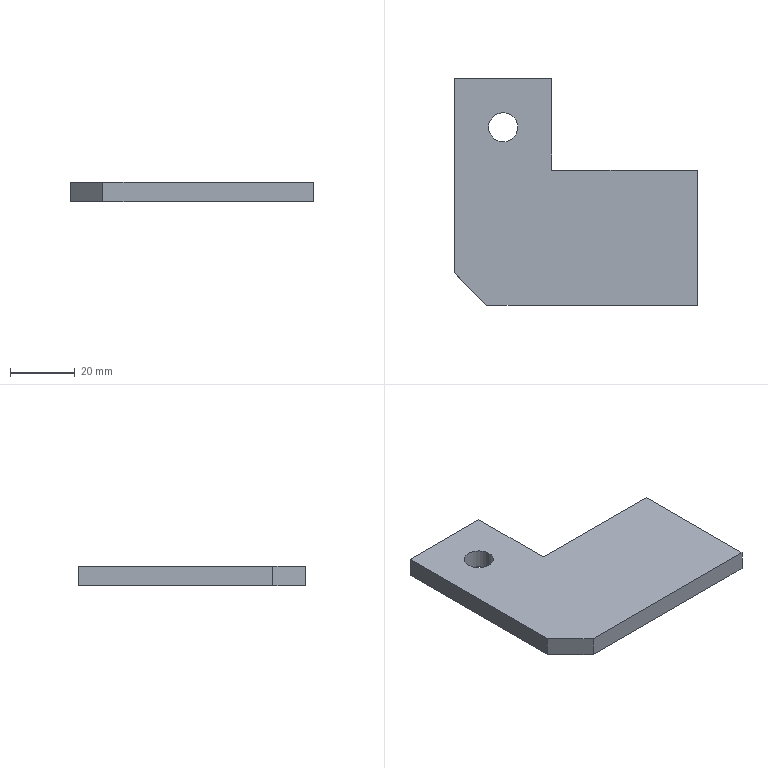Part | SolidWorks | features Chamfer 1, Extrusion 1, ICE 1 | 1 solid | 11 faces | box 75 x 70 x 6 mm | volume 23195 mm3 | plane 9 | cylinder 2 | commonest cylinder face diameters 9 x2
STEP:
#1=CARTESIAN_POINT('',(-23.022,36.378,0.));
#2=VERTEX_POINT('',#1);
#3=CARTESIAN_POINT('',(-14.022,36.378,0.));
#4=VERTEX_POINT('',#3);
#5=CARTESIAN_POINT('',(-18.522,36.378,0.));
#6=DIRECTION('',(0.,0.,1.));
#7=DIRECTION('',(-1.,0.,0.));
#8=AXIS2_PLACEMENT_3D('',#5,#6,#7);
#9=CIRCLE('',#8,4.5);
#10=EDGE_CURVE('',#2,#4,#9,.T.);
#11=ORIENTED_EDGE('',*,*,#10,.F.);
#12=CARTESIAN_POINT('',(-23.022,36.378,6.));
#13=VERTEX_POINT('',#12);
#14=CARTESIAN_POINT('',(-23.022,36.378,-0.001));
#15=DIRECTION('',(0.,0.,1.));
#16=VECTOR('',#15,1000.);
#17=LINE('',#14,#16);
#18=EDGE_CURVE('',#2,#13,#17,.T.);
#19=ORIENTED_EDGE('',*,*,#18,.T.);
#20=CARTESIAN_POINT('',(-14.022,36.378,6.));
#21=VERTEX_POINT('',#20);
#22=CARTESIAN_POINT('',(-18.522,36.378,6.));
#23=DIRECTION('',(0.,0.,1.));
#24=DIRECTION('',(1.,0.,0.));
#25=AXIS2_PLACEMENT_3D('',#22,#23,#24);
#26=CIRCLE('',#25,4.5);
#27=EDGE_CURVE('',#13,#21,#26,.T.);
#28=ORIENTED_EDGE('',*,*,#27,.T.);
#29=CARTESIAN_POINT('',(-14.022,36.378,-0.001));
#30=DIRECTION('',(0.,0.,1.));
#31=VECTOR('',#30,1000.);
#32=LINE('',#29,#31);
#33=EDGE_CURVE('',#4,#21,#32,.T.);
#34=ORIENTED_EDGE('',*,*,#33,.F.);
#35=EDGE_LOOP('',(#11,#19,#28,#34));
#36=FACE_OUTER_BOUND('',#35,.T.);
#37=CARTESIAN_POINT('',(-18.522,36.378,-0.001));
#38=DIRECTION('',(0.,0.,1.));
#39=DIRECTION('',(1.,0.,0.));
#40=AXIS2_PLACEMENT_3D('',#37,#38,#39);
#41=CYLINDRICAL_SURFACE('',#40,4.5);
#42=ADVANCED_FACE('',(#36),#41,.F.);
#43=CARTESIAN_POINT('',(-23.522,-18.622,6.));
#44=VERTEX_POINT('',#43);
#45=CARTESIAN_POINT('',(41.478,-18.622,6.));
#46=VERTEX_POINT('',#45);
#47=CARTESIAN_POINT('',(41.478,-18.622,6.));
#48=DIRECTION('',(1.,0.,0.));
#49=VECTOR('',#48,1000.);
#50=LINE('',#47,#49);
#51=EDGE_CURVE('',#44,#46,#50,.T.);
#52=ORIENTED_EDGE('',*,*,#51,.F.);
#53=CARTESIAN_POINT('',(-23.522,-18.622,0.));
#54=VERTEX_POINT('',#53);
#55=CARTESIAN_POINT('',(-23.522,-18.622,6.));
#56=DIRECTION('',(0.,0.,-1.));
#57=VECTOR('',#56,1000.);
#58=LINE('',#55,#57);
#59=EDGE_CURVE('',#44,#54,#58,.T.);
#60=ORIENTED_EDGE('',*,*,#59,.T.);
#61=CARTESIAN_POINT('',(41.478,-18.622,0.));
#62=VERTEX_POINT('',#61);
#63=CARTESIAN_POINT('',(41.478,-18.622,0.));
#64=DIRECTION('',(1.,0.,0.));
#65=VECTOR('',#64,1000.);
#66=LINE('',#63,#65);
#67=EDGE_CURVE('',#54,#62,#66,.T.);
#68=ORIENTED_EDGE('',*,*,#67,.T.);
#69=CARTESIAN_POINT('',(41.478,-18.622,6.));
#70=DIRECTION('',(0.,0.,-1.));
#71=VECTOR('',#70,1000.);
#72=LINE('',#69,#71);
#73=EDGE_CURVE('',#46,#62,#72,.T.);
#74=ORIENTED_EDGE('',*,*,#73,.F.);
#75=EDGE_LOOP('',(#52,#60,#68,#74));
#76=FACE_OUTER_BOUND('',#75,.T.);
#77=CARTESIAN_POINT('',(41.478,-18.622,6.));
#78=DIRECTION('',(0.,1.,0.));
#79=DIRECTION('',(-1.,0.,0.));
#80=AXIS2_PLACEMENT_3D('',#77,#78,#79);
#81=PLANE('',#80);
#82=ADVANCED_FACE('',(#76),#81,.F.);
#83=CARTESIAN_POINT('',(41.478,23.145,0.));
#84=VERTEX_POINT('',#83);
#85=CARTESIAN_POINT('',(41.478,23.145,0.));
#86=DIRECTION('',(0.,1.,0.));
#87=VECTOR('',#86,1000.);
#88=LINE('',#85,#87);
#89=EDGE_CURVE('',#62,#84,#88,.T.);
#90=ORIENTED_EDGE('',*,*,#89,.T.);
#91=CARTESIAN_POINT('',(41.478,23.145,6.));
#92=VERTEX_POINT('',#91);
#93=CARTESIAN_POINT('',(41.478,23.145,6.));
#94=DIRECTION('',(0.,0.,-1.));
#95=VECTOR('',#94,1000.);
#96=LINE('',#93,#95);
#97=EDGE_CURVE('',#92,#84,#96,.T.);
#98=ORIENTED_EDGE('',*,*,#97,.F.);
#99=CARTESIAN_POINT('',(41.478,23.145,6.));
#100=DIRECTION('',(0.,1.,0.));
#101=VECTOR('',#100,1000.);
#102=LINE('',#99,#101);
#103=EDGE_CURVE('',#46,#92,#102,.T.);
#104=ORIENTED_EDGE('',*,*,#103,.F.);
#105=ORIENTED_EDGE('',*,*,#73,.T.);
#106=EDGE_LOOP('',(#90,#98,#104,#105));
#107=FACE_OUTER_BOUND('',#106,.T.);
#108=CARTESIAN_POINT('',(41.478,23.145,6.));
#109=DIRECTION('',(-1.,0.,0.));
#110=DIRECTION('',(0.,0.,1.));
#111=AXIS2_PLACEMENT_3D('',#108,#109,#110);
#112=PLANE('',#111);
#113=ADVANCED_FACE('',(#107),#112,.F.);
#114=CARTESIAN_POINT('',(-3.522,23.145,0.));
#115=VERTEX_POINT('',#114);
#116=CARTESIAN_POINT('',(-3.522,23.145,0.));
#117=DIRECTION('',(-1.,0.,0.));
#118=VECTOR('',#117,1000.);
#119=LINE('',#116,#118);
#120=EDGE_CURVE('',#84,#115,#119,.T.);
#121=ORIENTED_EDGE('',*,*,#120,.T.);
#122=CARTESIAN_POINT('',(-3.522,23.145,6.));
#123=VERTEX_POINT('',#122);
#124=CARTESIAN_POINT('',(-3.522,23.145,6.));
#125=DIRECTION('',(0.,0.,-1.));
#126=VECTOR('',#125,1000.);
#127=LINE('',#124,#126);
#128=EDGE_CURVE('',#123,#115,#127,.T.);
#129=ORIENTED_EDGE('',*,*,#128,.F.);
#130=CARTESIAN_POINT('',(-3.522,23.145,6.));
#131=DIRECTION('',(-1.,0.,0.));
#132=VECTOR('',#131,1000.);
#133=LINE('',#130,#132);
#134=EDGE_CURVE('',#92,#123,#133,.T.);
#135=ORIENTED_EDGE('',*,*,#134,.F.);
#136=ORIENTED_EDGE('',*,*,#97,.T.);
#137=EDGE_LOOP('',(#121,#129,#135,#136));
#138=FACE_OUTER_BOUND('',#137,.T.);
#139=CARTESIAN_POINT('',(-3.522,23.145,6.));
#140=DIRECTION('',(0.,-1.,0.));
#141=DIRECTION('',(0.,0.,-1.));
#142=AXIS2_PLACEMENT_3D('',#139,#140,#141);
#143=PLANE('',#142);
#144=ADVANCED_FACE('',(#138),#143,.F.);
#145=CARTESIAN_POINT('',(-3.522,51.378,0.));
#146=VERTEX_POINT('',#145);
#147=CARTESIAN_POINT('',(-3.522,51.378,0.));
#148=DIRECTION('',(0.,1.,0.));
#149=VECTOR('',#148,1000.);
#150=LINE('',#147,#149);
#151=EDGE_CURVE('',#115,#146,#150,.T.);
#152=ORIENTED_EDGE('',*,*,#151,.T.);
#153=CARTESIAN_POINT('',(-3.522,51.378,6.));
#154=VERTEX_POINT('',#153);
#155=CARTESIAN_POINT('',(-3.522,51.378,6.));
#156=DIRECTION('',(0.,0.,-1.));
#157=VECTOR('',#156,1000.);
#158=LINE('',#155,#157);
#159=EDGE_CURVE('',#154,#146,#158,.T.);
#160=ORIENTED_EDGE('',*,*,#159,.F.);
#161=CARTESIAN_POINT('',(-3.522,51.378,6.));
#162=DIRECTION('',(0.,1.,0.));
#163=VECTOR('',#162,1000.);
#164=LINE('',#161,#163);
#165=EDGE_CURVE('',#123,#154,#164,.T.);
#166=ORIENTED_EDGE('',*,*,#165,.F.);
#167=ORIENTED_EDGE('',*,*,#128,.T.);
#168=EDGE_LOOP('',(#152,#160,#166,#167));
#169=FACE_OUTER_BOUND('',#168,.T.);
#170=CARTESIAN_POINT('',(-3.522,51.378,6.));
#171=DIRECTION('',(-1.,0.,0.));
#172=DIRECTION('',(0.,-1.,0.));
#173=AXIS2_PLACEMENT_3D('',#170,#171,#172);
#174=PLANE('',#173);
#175=ADVANCED_FACE('',(#169),#174,.F.);
#176=CARTESIAN_POINT('',(-33.522,51.378,0.));
#177=VERTEX_POINT('',#176);
#178=CARTESIAN_POINT('',(-33.522,51.378,0.));
#179=DIRECTION('',(-1.,0.,0.));
#180=VECTOR('',#179,1000.);
#181=LINE('',#178,#180);
#182=EDGE_CURVE('',#146,#177,#181,.T.);
#183=ORIENTED_EDGE('',*,*,#182,.T.);
#184=CARTESIAN_POINT('',(-33.522,51.378,6.));
#185=VERTEX_POINT('',#184);
#186=CARTESIAN_POINT('',(-33.522,51.378,6.));
#187=DIRECTION('',(0.,0.,-1.));
#188=VECTOR('',#187,1000.);
#189=LINE('',#186,#188);
#190=EDGE_CURVE('',#185,#177,#189,.T.);
#191=ORIENTED_EDGE('',*,*,#190,.F.);
#192=CARTESIAN_POINT('',(-33.522,51.378,6.));
#193=DIRECTION('',(-1.,0.,0.));
#194=VECTOR('',#193,1000.);
#195=LINE('',#192,#194);
#196=EDGE_CURVE('',#154,#185,#195,.T.);
#197=ORIENTED_EDGE('',*,*,#196,.F.);
#198=ORIENTED_EDGE('',*,*,#159,.T.);
#199=EDGE_LOOP('',(#183,#191,#197,#198));
#200=FACE_OUTER_BOUND('',#199,.T.);
#201=CARTESIAN_POINT('',(-33.522,51.378,6.));
#202=DIRECTION('',(0.,-1.,0.));
#203=DIRECTION('',(0.,0.,-1.));
#204=AXIS2_PLACEMENT_3D('',#201,#202,#203);
#205=PLANE('',#204);
#206=ADVANCED_FACE('',(#200),#205,.F.);
#207=CARTESIAN_POINT('',(-33.522,-8.622,0.));
#208=VERTEX_POINT('',#207);
#209=CARTESIAN_POINT('',(-33.522,-18.622,0.));
#210=DIRECTION('',(0.,-1.,0.));
#211=VECTOR('',#210,1000.);
#212=LINE('',#209,#211);
#213=EDGE_CURVE('',#177,#208,#212,.T.);
#214=ORIENTED_EDGE('',*,*,#213,.T.);
#215=CARTESIAN_POINT('',(-33.522,-8.622,6.));
#216=VERTEX_POINT('',#215);
#217=CARTESIAN_POINT('',(-33.522,-8.622,6.));
#218=DIRECTION('',(0.,0.,1.));
#219=VECTOR('',#218,1000.);
#220=LINE('',#217,#219);
#221=EDGE_CURVE('',#208,#216,#220,.T.);
#222=ORIENTED_EDGE('',*,*,#221,.T.);
#223=CARTESIAN_POINT('',(-33.522,-18.622,6.));
#224=DIRECTION('',(0.,-1.,0.));
#225=VECTOR('',#224,1000.);
#226=LINE('',#223,#225);
#227=EDGE_CURVE('',#185,#216,#226,.T.);
#228=ORIENTED_EDGE('',*,*,#227,.F.);
#229=ORIENTED_EDGE('',*,*,#190,.T.);
#230=EDGE_LOOP('',(#214,#222,#228,#229));
#231=FACE_OUTER_BOUND('',#230,.T.);
#232=CARTESIAN_POINT('',(-33.522,-18.622,6.));
#233=DIRECTION('',(1.,0.,0.));
#234=DIRECTION('',(0.,0.,-1.));
#235=AXIS2_PLACEMENT_3D('',#232,#233,#234);
#236=PLANE('',#235);
#237=ADVANCED_FACE('',(#231),#236,.F.);
#238=CARTESIAN_POINT('',(-18.522,36.378,6.));
#239=DIRECTION('',(0.,0.,1.));
#240=DIRECTION('',(1.,0.,0.));
#241=AXIS2_PLACEMENT_3D('',#238,#239,#240);
#242=CIRCLE('',#241,4.5);
#243=EDGE_CURVE('',#21,#13,#242,.T.);
#244=ORIENTED_EDGE('',*,*,#243,.F.);
#245=ORIENTED_EDGE('',*,*,#27,.F.);
#246=EDGE_LOOP('',(#244,#245));
#247=FACE_BOUND('',#246,.T.);
#248=ORIENTED_EDGE('',*,*,#227,.T.);
#249=CARTESIAN_POINT('',(-23.522,-18.622,6.));
#250=DIRECTION('',(0.7071,-0.7071,0.));
#251=VECTOR('',#250,1000.);
#252=LINE('',#249,#251);
#253=EDGE_CURVE('',#216,#44,#252,.T.);
#254=ORIENTED_EDGE('',*,*,#253,.T.);
#255=ORIENTED_EDGE('',*,*,#51,.T.);
#256=ORIENTED_EDGE('',*,*,#103,.T.);
#257=ORIENTED_EDGE('',*,*,#134,.T.);
#258=ORIENTED_EDGE('',*,*,#165,.T.);
#259=ORIENTED_EDGE('',*,*,#196,.T.);
#260=EDGE_LOOP('',(#248,#254,#255,#256,#257,#258,#259));
#261=FACE_OUTER_BOUND('',#260,.T.);
#262=CARTESIAN_POINT('',(0.,0.,6.));
#263=DIRECTION('',(0.,0.,-1.));
#264=DIRECTION('',(-1.,0.,0.));
#265=AXIS2_PLACEMENT_3D('',#262,#263,#264);
#266=PLANE('',#265);
#267=ADVANCED_FACE('',(#247,#261),#266,.F.);
#268=CARTESIAN_POINT('',(-18.522,36.378,0.));
#269=DIRECTION('',(0.,0.,1.));
#270=DIRECTION('',(-1.,0.,0.));
#271=AXIS2_PLACEMENT_3D('',#268,#269,#270);
#272=CIRCLE('',#271,4.5);
#273=EDGE_CURVE('',#4,#2,#272,.T.);
#274=ORIENTED_EDGE('',*,*,#273,.T.);
#275=ORIENTED_EDGE('',*,*,#10,.T.);
#276=EDGE_LOOP('',(#274,#275));
#277=FACE_BOUND('',#276,.T.);
#278=ORIENTED_EDGE('',*,*,#67,.F.);
#279=CARTESIAN_POINT('',(-21.072,-21.072,0.));
#280=DIRECTION('',(-0.7071,0.7071,0.));
#281=VECTOR('',#280,1000.);
#282=LINE('',#279,#281);
#283=EDGE_CURVE('',#54,#208,#282,.T.);
#284=ORIENTED_EDGE('',*,*,#283,.T.);
#285=ORIENTED_EDGE('',*,*,#213,.F.);
#286=ORIENTED_EDGE('',*,*,#182,.F.);
#287=ORIENTED_EDGE('',*,*,#151,.F.);
#288=ORIENTED_EDGE('',*,*,#120,.F.);
#289=ORIENTED_EDGE('',*,*,#89,.F.);
#290=EDGE_LOOP('',(#278,#284,#285,#286,#287,#288,#289));
#291=FACE_OUTER_BOUND('',#290,.T.);
#292=CARTESIAN_POINT('',(0.,0.,0.));
#293=DIRECTION('',(0.,0.,-1.));
#294=DIRECTION('',(-1.,0.,0.));
#295=AXIS2_PLACEMENT_3D('',#292,#293,#294);
#296=PLANE('',#295);
#297=ADVANCED_FACE('',(#277,#291),#296,.T.);
#298=ORIENTED_EDGE('',*,*,#18,.F.);
#299=ORIENTED_EDGE('',*,*,#273,.F.);
#300=ORIENTED_EDGE('',*,*,#33,.T.);
#301=ORIENTED_EDGE('',*,*,#243,.T.);
#302=EDGE_LOOP('',(#298,#299,#300,#301));
#303=FACE_OUTER_BOUND('',#302,.T.);
#304=CARTESIAN_POINT('',(-18.522,36.378,-0.001));
#305=DIRECTION('',(0.,0.,1.));
#306=DIRECTION('',(1.,0.,0.));
#307=AXIS2_PLACEMENT_3D('',#304,#305,#306);
#308=CYLINDRICAL_SURFACE('',#307,4.5);
#309=ADVANCED_FACE('',(#303),#308,.F.);
#310=ORIENTED_EDGE('',*,*,#253,.F.);
#311=ORIENTED_EDGE('',*,*,#221,.F.);
#312=ORIENTED_EDGE('',*,*,#283,.F.);
#313=ORIENTED_EDGE('',*,*,#59,.F.);
#314=EDGE_LOOP('',(#310,#311,#312,#313));
#315=FACE_OUTER_BOUND('',#314,.T.);
#316=CARTESIAN_POINT('',(-23.522,-18.622,6.));
#317=DIRECTION('',(0.7071,0.7071,0.));
#318=DIRECTION('',(0.,0.,-1.));
#319=AXIS2_PLACEMENT_3D('',#316,#317,#318);
#320=PLANE('',#319);
#321=ADVANCED_FACE('',(#315),#320,.F.);
#322=CLOSED_SHELL('',(#42,#82,#113,#144,#175,#206,#237,#267,#297,#309,#321));
#323=MANIFOLD_SOLID_BREP('',#322);
#324=CARTESIAN_POINT('',(0.,0.,0.));
#325=DIRECTION('',(0.,0.,1.));
#326=DIRECTION('',(1.,0.,0.));
#327=AXIS2_PLACEMENT_3D('',#324,#325,#326);
#328=(LENGTH_UNIT()NAMED_UNIT(*)SI_UNIT(.MILLI.,.METRE.));
#329=UNCERTAINTY_MEASURE_WITH_UNIT(LENGTH_MEASURE(0.00001),#328,'','');
#330=(NAMED_UNIT(*)PLANE_ANGLE_UNIT()SI_UNIT($,.RADIAN.));
#331=(NAMED_UNIT(*)SI_UNIT($,.STERADIAN.)SOLID_ANGLE_UNIT());
#332=(GEOMETRIC_REPRESENTATION_CONTEXT(3)GLOBAL_UNCERTAINTY_ASSIGNED_CONTEXT((#329))GLOBAL_UNIT_ASSIGNED_CONTEXT((#328,#330,#331))REPRESENTATION_CONTEXT('',''));
#333=ADVANCED_BREP_SHAPE_REPRESENTATION('',(#323,#327),#332);